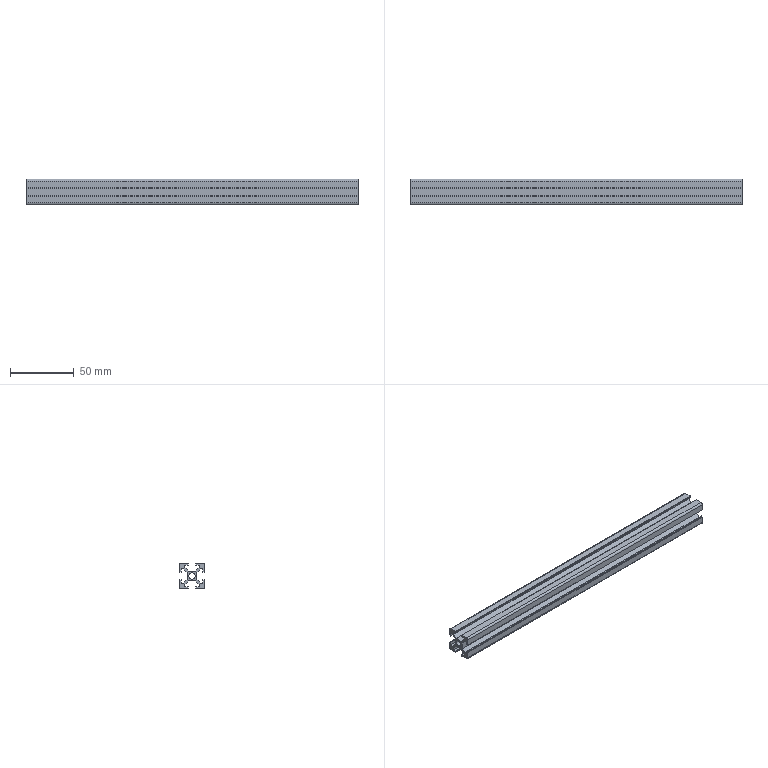Part | SolidWorks | features WeldMemberFeat 1, WeldmentFeature 1 | 1 solid | 68 faces | box 260 x 20 x 20 mm | volume 43442 mm3 | plane 62 | cylinder 6 | commonest cylinder face diameters 3 x4 5 x2